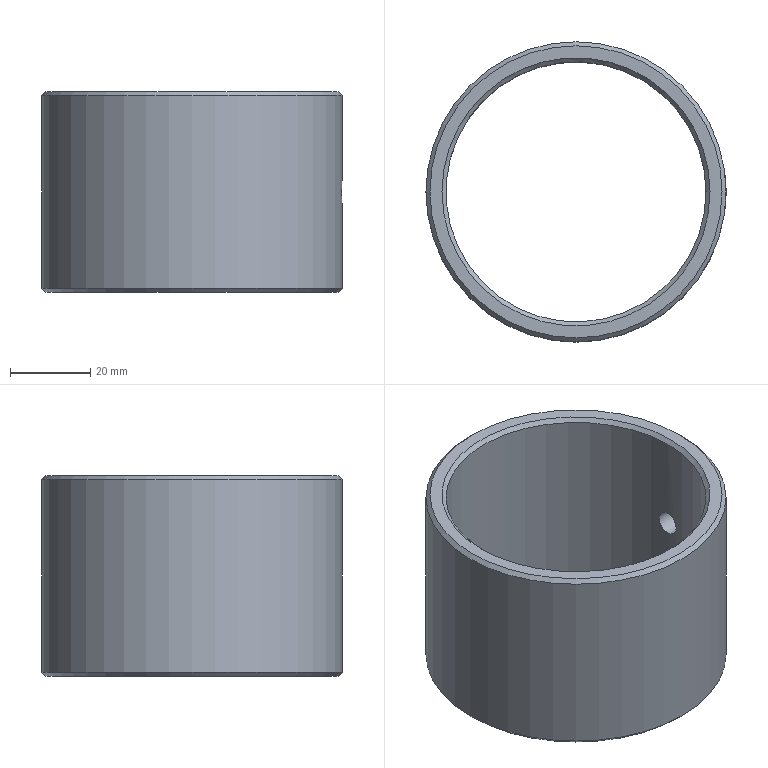Part | NX | features DATUM_CSYS 3, EXTRUDE 2, SKETCH 2, CHAMFER 1 | 1 solid | 9 faces | box 75 x 75 x 50 mm | volume 54397 mm3 | cone 4 | cylinder 3 | plane 2 | commonest cylinder face diameters 6 x1 65 x1 75 x1
STEP:
#1=CARTESIAN_POINT('',(37.5,0.,1.));
#2=VERTEX_POINT('',#1);
#3=CARTESIAN_POINT('',(0.,0.,1.));
#4=DIRECTION('',(0.,0.,1.));
#5=DIRECTION('',(1.,0.,0.));
#6=AXIS2_PLACEMENT_3D('',#3,#4,#5);
#7=CIRCLE('',#6,37.5);
#8=EDGE_CURVE('',#2,#2,#7,.T.);
#9=ORIENTED_EDGE('',*,*,#8,.T.);
#10=EDGE_LOOP('',(#9));
#11=FACE_BOUND('',#10,.T.);
#12=CARTESIAN_POINT('',(37.5,0.,49.));
#13=VERTEX_POINT('',#12);
#14=CARTESIAN_POINT('',(0.,0.,49.));
#15=DIRECTION('',(0.,0.,1.));
#16=DIRECTION('',(1.,0.,0.));
#17=AXIS2_PLACEMENT_3D('',#14,#15,#16);
#18=CIRCLE('',#17,37.5);
#19=EDGE_CURVE('',#13,#13,#18,.F.);
#20=ORIENTED_EDGE('',*,*,#19,.T.);
#21=EDGE_LOOP('',(#20));
#22=FACE_BOUND('',#21,.T.);
#23=CARTESIAN_POINT('',(37.5,0.,28.));
#24=VERTEX_POINT('',#23);
#25=CARTESIAN_POINT('',(37.44,2.353,27.349));
#26=CARTESIAN_POINT('',(37.53,-0.0005947,28.325));
#27=CARTESIAN_POINT('',(37.44,-2.351,27.35));
#28=CARTESIAN_POINT('',(37.35,-3.324,25.003));
#29=CARTESIAN_POINT('',(37.44,-2.352,22.65));
#30=CARTESIAN_POINT('',(37.53,-0.0005291,21.676));
#31=CARTESIAN_POINT('',(37.44,2.348,22.647));
#32=CARTESIAN_POINT('',(37.35,3.325,24.997));
#33=CARTESIAN_POINT('',(37.44,2.353,27.349));
#34=CARTESIAN_POINT('',(37.53,-0.0005947,28.325));
#35=CARTESIAN_POINT('',(37.44,-2.351,27.35));
#36=B_SPLINE_CURVE_WITH_KNOTS('',3,(#25,#26,#27,#28,#29,#30,#31,#32,#33,#34,#35),.UNSPECIFIED.,.T.,.F.,(1,1,1,1,1,1,1,1,1,1,1,1,1,1,1),(-0.007037,-0.004691,-0.002346,0.,0.002346,0.004691,0.007037,0.009382,0.01173,0.01407,0.01642,0.01876,0.02111,0.02346,0.0258),.UNSPECIFIED.);
#37=EDGE_CURVE('',#24,#24,#36,.T.);
#38=ORIENTED_EDGE('',*,*,#37,.F.);
#39=EDGE_LOOP('',(#38));
#40=FACE_BOUND('',#39,.T.);
#41=CARTESIAN_POINT('',(0.,0.,50.));
#42=DIRECTION('',(0.,0.,-1.));
#43=DIRECTION('',(-1.,0.,0.));
#44=AXIS2_PLACEMENT_3D('',#41,#42,#43);
#45=CYLINDRICAL_SURFACE('',#44,37.5);
#46=ADVANCED_FACE('',(#11,#22,#40),#45,.T.);
#47=CARTESIAN_POINT('',(32.5,0.,1.));
#48=VERTEX_POINT('',#47);
#49=CARTESIAN_POINT('',(0.,0.,1.));
#50=DIRECTION('',(0.,0.,1.));
#51=DIRECTION('',(1.,0.,0.));
#52=AXIS2_PLACEMENT_3D('',#49,#50,#51);
#53=CIRCLE('',#52,32.5);
#54=EDGE_CURVE('',#48,#48,#53,.F.);
#55=ORIENTED_EDGE('',*,*,#54,.T.);
#56=EDGE_LOOP('',(#55));
#57=FACE_BOUND('',#56,.T.);
#58=CARTESIAN_POINT('',(32.5,0.,49.));
#59=VERTEX_POINT('',#58);
#60=CARTESIAN_POINT('',(0.,0.,49.));
#61=DIRECTION('',(0.,0.,1.));
#62=DIRECTION('',(1.,0.,0.));
#63=AXIS2_PLACEMENT_3D('',#60,#61,#62);
#64=CIRCLE('',#63,32.5);
#65=EDGE_CURVE('',#59,#59,#64,.T.);
#66=ORIENTED_EDGE('',*,*,#65,.T.);
#67=EDGE_LOOP('',(#66));
#68=FACE_BOUND('',#67,.T.);
#69=CARTESIAN_POINT('',(32.5,0.,28.));
#70=VERTEX_POINT('',#69);
#71=CARTESIAN_POINT('',(32.431,2.353,27.349));
#72=CARTESIAN_POINT('',(32.535,-0.0005914,28.325));
#73=CARTESIAN_POINT('',(32.431,-2.351,27.35));
#74=CARTESIAN_POINT('',(32.327,-3.324,25.003));
#75=CARTESIAN_POINT('',(32.431,-2.352,22.65));
#76=CARTESIAN_POINT('',(32.535,-0.0005633,21.676));
#77=CARTESIAN_POINT('',(32.431,2.348,22.647));
#78=CARTESIAN_POINT('',(32.326,3.325,24.997));
#79=CARTESIAN_POINT('',(32.431,2.353,27.349));
#80=CARTESIAN_POINT('',(32.535,-0.0005914,28.325));
#81=CARTESIAN_POINT('',(32.431,-2.351,27.35));
#82=B_SPLINE_CURVE_WITH_KNOTS('',3,(#71,#72,#73,#74,#75,#76,#77,#78,#79,#80,#81),.UNSPECIFIED.,.T.,.F.,(1,1,1,1,1,1,1,1,1,1,1,1,1,1,1),(-0.007037,-0.004692,-0.002346,0.,0.002346,0.004692,0.007037,0.009383,0.01173,0.01407,0.01642,0.01877,0.02111,0.02346,0.0258),.UNSPECIFIED.);
#83=EDGE_CURVE('',#70,#70,#82,.T.);
#84=ORIENTED_EDGE('',*,*,#83,.T.);
#85=EDGE_LOOP('',(#84));
#86=FACE_BOUND('',#85,.T.);
#87=CARTESIAN_POINT('',(0.,0.,50.));
#88=DIRECTION('',(0.,0.,-1.));
#89=DIRECTION('',(-1.,0.,0.));
#90=AXIS2_PLACEMENT_3D('',#87,#88,#89);
#91=CYLINDRICAL_SURFACE('',#90,32.5);
#92=ADVANCED_FACE('',(#57,#68,#86),#91,.F.);
#93=CARTESIAN_POINT('',(36.5,0.,50.));
#94=VERTEX_POINT('',#93);
#95=CARTESIAN_POINT('',(0.,0.,50.));
#96=DIRECTION('',(0.,0.,1.));
#97=DIRECTION('',(1.,0.,0.));
#98=AXIS2_PLACEMENT_3D('',#95,#96,#97);
#99=CIRCLE('',#98,36.5);
#100=EDGE_CURVE('',#94,#94,#99,.T.);
#101=ORIENTED_EDGE('',*,*,#100,.T.);
#102=EDGE_LOOP('',(#101));
#103=FACE_BOUND('',#102,.T.);
#104=CARTESIAN_POINT('',(33.5,0.,50.));
#105=VERTEX_POINT('',#104);
#106=CARTESIAN_POINT('',(0.,0.,50.));
#107=DIRECTION('',(0.,0.,1.));
#108=DIRECTION('',(1.,0.,0.));
#109=AXIS2_PLACEMENT_3D('',#106,#107,#108);
#110=CIRCLE('',#109,33.5);
#111=EDGE_CURVE('',#105,#105,#110,.F.);
#112=ORIENTED_EDGE('',*,*,#111,.T.);
#113=EDGE_LOOP('',(#112));
#114=FACE_BOUND('',#113,.T.);
#115=CARTESIAN_POINT('',(0.,0.,50.));
#116=DIRECTION('',(0.,0.,1.));
#117=DIRECTION('',(1.,0.,0.));
#118=AXIS2_PLACEMENT_3D('',#115,#116,#117);
#119=PLANE('',#118);
#120=ADVANCED_FACE('',(#103,#114),#119,.T.);
#121=CARTESIAN_POINT('',(36.5,0.,0.));
#122=VERTEX_POINT('',#121);
#123=CARTESIAN_POINT('',(0.,0.,0.));
#124=DIRECTION('',(0.,0.,1.));
#125=DIRECTION('',(1.,0.,0.));
#126=AXIS2_PLACEMENT_3D('',#123,#124,#125);
#127=CIRCLE('',#126,36.5);
#128=EDGE_CURVE('',#122,#122,#127,.F.);
#129=ORIENTED_EDGE('',*,*,#128,.T.);
#130=EDGE_LOOP('',(#129));
#131=FACE_BOUND('',#130,.T.);
#132=CARTESIAN_POINT('',(33.5,0.,0.));
#133=VERTEX_POINT('',#132);
#134=CARTESIAN_POINT('',(0.,0.,0.));
#135=DIRECTION('',(0.,0.,1.));
#136=DIRECTION('',(1.,0.,0.));
#137=AXIS2_PLACEMENT_3D('',#134,#135,#136);
#138=CIRCLE('',#137,33.5);
#139=EDGE_CURVE('',#133,#133,#138,.T.);
#140=ORIENTED_EDGE('',*,*,#139,.T.);
#141=EDGE_LOOP('',(#140));
#142=FACE_BOUND('',#141,.T.);
#143=CARTESIAN_POINT('',(0.,0.,0.));
#144=DIRECTION('',(0.,0.,1.));
#145=DIRECTION('',(1.,0.,0.));
#146=AXIS2_PLACEMENT_3D('',#143,#144,#145);
#147=PLANE('',#146);
#148=ADVANCED_FACE('',(#131,#142),#147,.F.);
#149=ORIENTED_EDGE('',*,*,#83,.F.);
#150=EDGE_LOOP('',(#149));
#151=FACE_BOUND('',#150,.T.);
#152=ORIENTED_EDGE('',*,*,#37,.T.);
#153=EDGE_LOOP('',(#152));
#154=FACE_BOUND('',#153,.T.);
#155=CARTESIAN_POINT('',(50.,0.,25.));
#156=DIRECTION('',(-1.,0.,0.));
#157=DIRECTION('',(0.,0.,1.));
#158=AXIS2_PLACEMENT_3D('',#155,#156,#157);
#159=CYLINDRICAL_SURFACE('',#158,3.);
#160=ADVANCED_FACE('',(#151,#154),#159,.F.);
#161=ORIENTED_EDGE('',*,*,#128,.F.);
#162=EDGE_LOOP('',(#161));
#163=FACE_BOUND('',#162,.T.);
#164=ORIENTED_EDGE('',*,*,#8,.F.);
#165=EDGE_LOOP('',(#164));
#166=FACE_BOUND('',#165,.T.);
#167=CARTESIAN_POINT('',(0.,0.,1.));
#168=DIRECTION('',(0.,0.,1.));
#169=DIRECTION('',(1.,0.,0.));
#170=AXIS2_PLACEMENT_3D('',#167,#168,#169);
#171=CONICAL_SURFACE('',#170,37.5,0.7854);
#172=ADVANCED_FACE('',(#163,#166),#171,.T.);
#173=ORIENTED_EDGE('',*,*,#54,.F.);
#174=EDGE_LOOP('',(#173));
#175=FACE_BOUND('',#174,.T.);
#176=ORIENTED_EDGE('',*,*,#139,.F.);
#177=EDGE_LOOP('',(#176));
#178=FACE_BOUND('',#177,.T.);
#179=CARTESIAN_POINT('',(0.,0.,0.));
#180=DIRECTION('',(0.,0.,-1.));
#181=DIRECTION('',(-1.,0.,0.));
#182=AXIS2_PLACEMENT_3D('',#179,#180,#181);
#183=CONICAL_SURFACE('',#182,33.5,0.7854);
#184=ADVANCED_FACE('',(#175,#178),#183,.F.);
#185=ORIENTED_EDGE('',*,*,#19,.F.);
#186=EDGE_LOOP('',(#185));
#187=FACE_BOUND('',#186,.T.);
#188=ORIENTED_EDGE('',*,*,#100,.F.);
#189=EDGE_LOOP('',(#188));
#190=FACE_BOUND('',#189,.T.);
#191=CARTESIAN_POINT('',(0.,0.,50.));
#192=DIRECTION('',(0.,0.,-1.));
#193=DIRECTION('',(-1.,0.,0.));
#194=AXIS2_PLACEMENT_3D('',#191,#192,#193);
#195=CONICAL_SURFACE('',#194,36.5,0.7854);
#196=ADVANCED_FACE('',(#187,#190),#195,.T.);
#197=ORIENTED_EDGE('',*,*,#111,.F.);
#198=EDGE_LOOP('',(#197));
#199=FACE_BOUND('',#198,.T.);
#200=ORIENTED_EDGE('',*,*,#65,.F.);
#201=EDGE_LOOP('',(#200));
#202=FACE_BOUND('',#201,.T.);
#203=CARTESIAN_POINT('',(0.,0.,49.));
#204=DIRECTION('',(0.,0.,1.));
#205=DIRECTION('',(1.,0.,0.));
#206=AXIS2_PLACEMENT_3D('',#203,#204,#205);
#207=CONICAL_SURFACE('',#206,32.5,0.7854);
#208=ADVANCED_FACE('',(#199,#202),#207,.F.);
#209=CLOSED_SHELL('',(#46,#92,#120,#148,#160,#172,#184,#196,#208));
#210=MANIFOLD_SOLID_BREP('',#209);
#211=(LENGTH_UNIT()NAMED_UNIT(*)SI_UNIT(.MILLI.,.METRE.));
#212=UNCERTAINTY_MEASURE_WITH_UNIT(LENGTH_MEASURE(0.0508),#211,'','');
#213=(NAMED_UNIT(*)PLANE_ANGLE_UNIT()SI_UNIT($,.RADIAN.));
#214=(NAMED_UNIT(*)SI_UNIT($,.STERADIAN.)SOLID_ANGLE_UNIT());
#215=(GEOMETRIC_REPRESENTATION_CONTEXT(3)GLOBAL_UNCERTAINTY_ASSIGNED_CONTEXT((#212))GLOBAL_UNIT_ASSIGNED_CONTEXT((#211,#213,#214))REPRESENTATION_CONTEXT('',''));
#216=ADVANCED_BREP_SHAPE_REPRESENTATION('',(#210),#215);